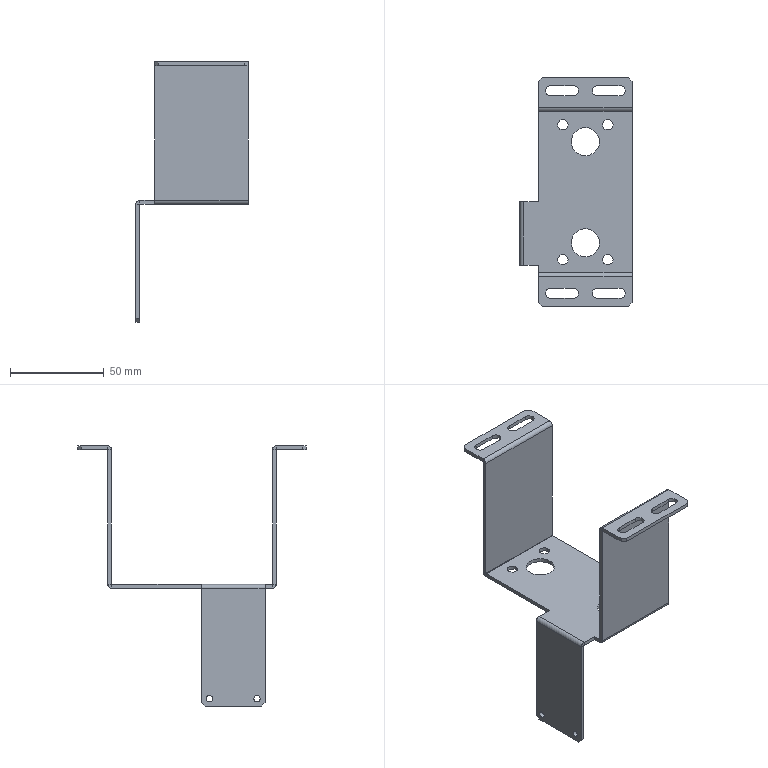Part | STEP file | 1 solid | 92 faces | box 60 x 122 x 139 mm | volume 30068 mm3 | plane 54 | cylinder 38 | commonest cylinder face diameters 5.5 x20 0.2 x5 4.2 x5 3.4 x4 15 x4